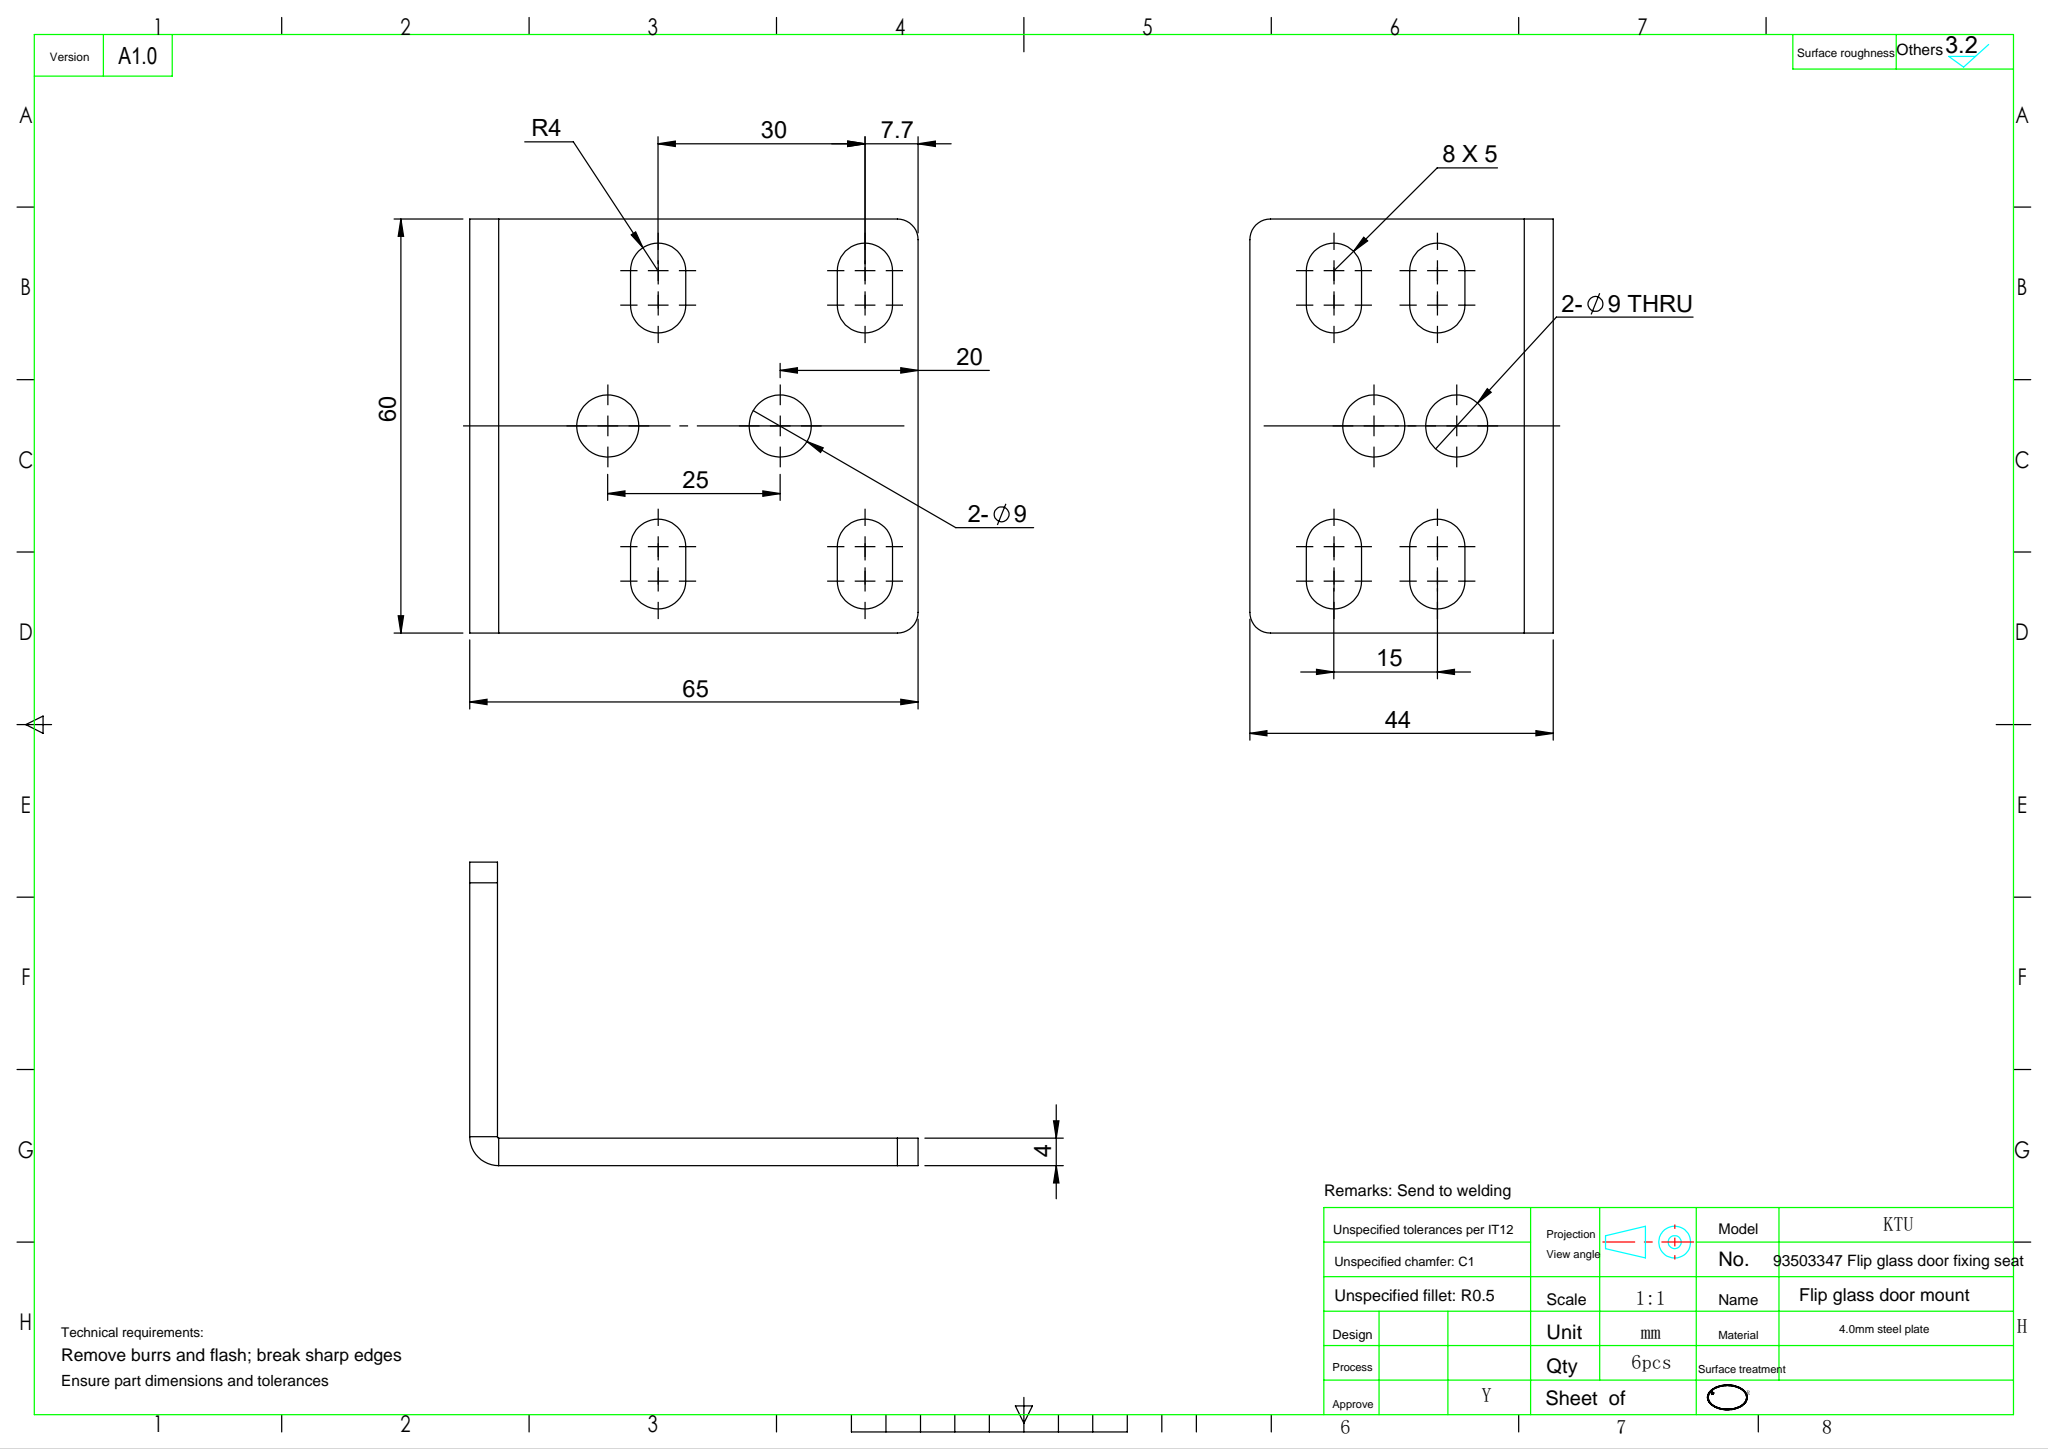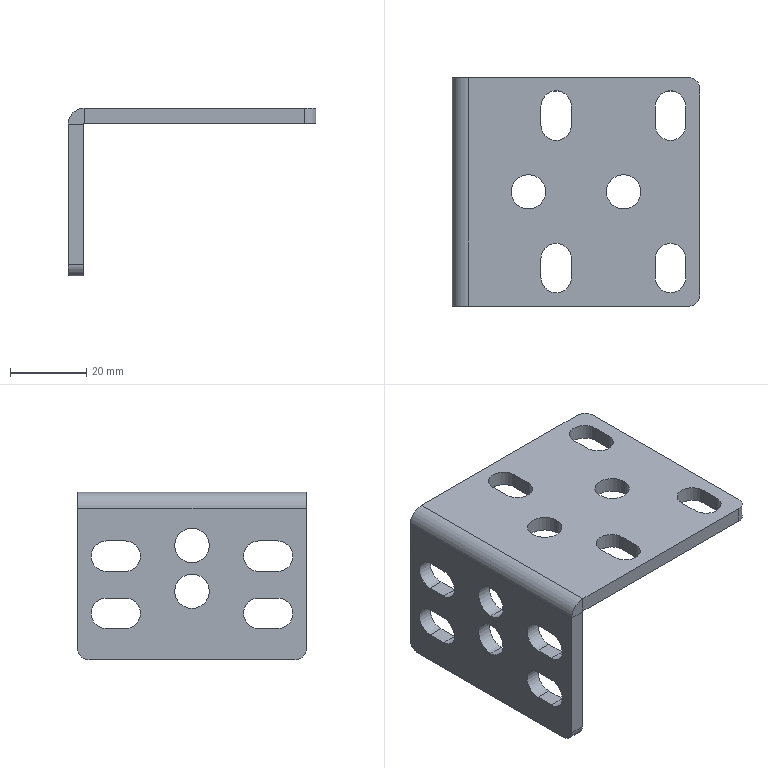Part | SolidWorks | features ICE 4, Fillet 1, FlatPattern 1, SMBaseFlange 1, SheetMetal 1 | 1 solid | 58 faces | box 65 x 60 x 44 mm | volume 21036 mm3 | cylinder 30 | plane 28 | commonest cylinder face diameters 8 x16 9 x8 6 x4 0.4 x1 8.4 x1